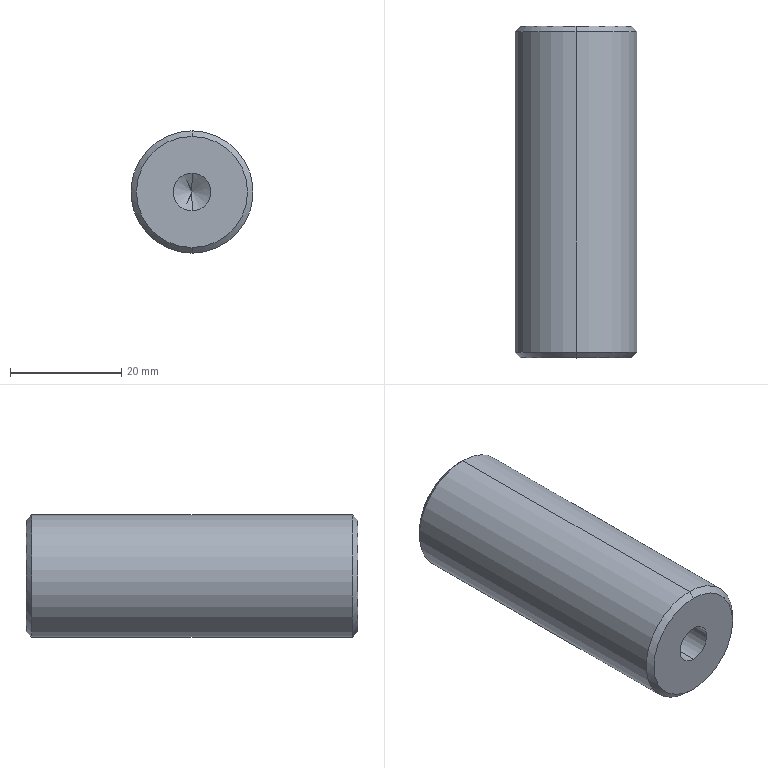Part | STEP file | circular post spca dia22-16-M8 | 1 solid | 16 faces | box 22 x 59.7 x 22 mm | volume 21361 mm3 | cone 8 | cylinder 6 | plane 2 | commonest cylinder face diameters 6.8 x4 22 x2
STEP:
#1=CARTESIAN_POINT('',(0.,0.,0.));
#2=DIRECTION('',(0.,0.,1.));
#3=DIRECTION('',(1.,0.,0.));
#4=AXIS2_PLACEMENT_3D('',#1,#2,#3);
#5=CARTESIAN_POINT('',(0.,0.,-10.));
#6=VERTEX_POINT('',#5);
#7=CARTESIAN_POINT('',(0.,0.,10.));
#8=VERTEX_POINT('',#7);
#9=CARTESIAN_POINT('',(0.,0.,0.));
#10=DIRECTION('',(0.,-1.,0.));
#11=DIRECTION('',(0.,0.,1.));
#12=AXIS2_PLACEMENT_3D('',#9,#10,#11);
#13=CIRCLE('',#12,10.);
#14=CARTESIAN_POINT('',(0.,1.,0.));
#15=DIRECTION('',(0.,1.,0.));
#16=DIRECTION('',(0.,0.,1.));
#17=AXIS2_PLACEMENT_3D('',#14,#15,#16);
#18=CONICAL_SURFACE('',#17,11.,0.7854);
#19=CARTESIAN_POINT('',(6.283,-1.));
#20=DIRECTION('',(-1.,0.));
#21=VECTOR('',#20,1.);
#22=LINE('',#19,#21);
#23=(GEOMETRIC_REPRESENTATION_CONTEXT(2)PARAMETRIC_REPRESENTATION_CONTEXT()REPRESENTATION_CONTEXT('',''));
#24=DEFINITIONAL_REPRESENTATION('',(#22),#23);
#25=PCURVE('',#18,#24);
#26=CARTESIAN_POINT('',(0.,0.,0.));
#27=DIRECTION('',(0.,1.,0.));
#28=DIRECTION('',(0.,0.,1.));
#29=AXIS2_PLACEMENT_3D('',#26,#27,#28);
#30=PLANE('',#29);
#31=CARTESIAN_POINT('',(10.,0.));
#32=CARTESIAN_POINT('',(10.,-17.321));
#33=CARTESIAN_POINT('',(-5.,-8.66));
#34=CARTESIAN_POINT('',(-20.,0.));
#35=CARTESIAN_POINT('',(-5.,8.66));
#36=CARTESIAN_POINT('',(10.,17.321));
#37=CARTESIAN_POINT('',(10.,0.));
#38=(BOUNDED_CURVE()B_SPLINE_CURVE(2,(#31,#32,#33,#34,#35,#36,#37),.UNSPECIFIED.,.T.,.F.)B_SPLINE_CURVE_WITH_KNOTS((1,2,2,2,2,1),(-2.094,0.,2.094,4.189,6.283,8.378),.UNSPECIFIED.)CURVE()GEOMETRIC_REPRESENTATION_ITEM()RATIONAL_B_SPLINE_CURVE((1.,0.5,1.,0.5,1.,0.5,1.))REPRESENTATION_ITEM(''));
#39=(GEOMETRIC_REPRESENTATION_CONTEXT(2)PARAMETRIC_REPRESENTATION_CONTEXT()REPRESENTATION_CONTEXT('',''));
#40=DEFINITIONAL_REPRESENTATION('',(#38),#39);
#41=PCURVE('',#30,#40);
#42=SURFACE_CURVE('',#13,(#25,#41),.PCURVE_S1.);
#43=EDGE_CURVE('',#6,#8,#42,.T.);
#44=ORIENTED_EDGE('',*,*,#43,.F.);
#45=CARTESIAN_POINT('',(0.,1.,-11.));
#46=VERTEX_POINT('',#45);
#47=CARTESIAN_POINT('',(0.,1.,-11.));
#48=DIRECTION('',(0.,0.7071,-0.7071));
#49=VECTOR('',#48,1.);
#50=LINE('',#47,#49);
#51=CARTESIAN_POINT('',(3.142,0.));
#52=DIRECTION('',(0.,1.));
#53=VECTOR('',#52,1.);
#54=LINE('',#51,#53);
#55=(GEOMETRIC_REPRESENTATION_CONTEXT(2)PARAMETRIC_REPRESENTATION_CONTEXT()REPRESENTATION_CONTEXT('',''));
#56=DEFINITIONAL_REPRESENTATION('',(#54),#55);
#57=PCURVE('',#18,#56);
#58=CARTESIAN_POINT('',(0.,1.,0.));
#59=DIRECTION('',(0.,1.,0.));
#60=DIRECTION('',(0.,0.,1.));
#61=AXIS2_PLACEMENT_3D('',#58,#59,#60);
#62=CONICAL_SURFACE('',#61,11.,0.7854);
#63=CARTESIAN_POINT('',(3.142,0.));
#64=DIRECTION('',(0.,1.));
#65=VECTOR('',#64,1.);
#66=LINE('',#63,#65);
#67=(GEOMETRIC_REPRESENTATION_CONTEXT(2)PARAMETRIC_REPRESENTATION_CONTEXT()REPRESENTATION_CONTEXT('',''));
#68=DEFINITIONAL_REPRESENTATION('',(#66),#67);
#69=PCURVE('',#62,#68);
#70=SURFACE_CURVE('',#50,(#57,#69),.PCURVE_S1.);
#71=EDGE_CURVE('',#6,#46,#70,.T.);
#72=ORIENTED_EDGE('',*,*,#71,.T.);
#73=CARTESIAN_POINT('',(0.,1.,11.));
#74=VERTEX_POINT('',#73);
#75=CARTESIAN_POINT('',(0.,1.,0.));
#76=DIRECTION('',(0.,1.,0.));
#77=DIRECTION('',(0.,0.,1.));
#78=AXIS2_PLACEMENT_3D('',#75,#76,#77);
#79=CIRCLE('',#78,11.);
#80=CARTESIAN_POINT('',(0.,0.));
#81=DIRECTION('',(1.,0.));
#82=VECTOR('',#81,1.);
#83=LINE('',#80,#82);
#84=(GEOMETRIC_REPRESENTATION_CONTEXT(2)PARAMETRIC_REPRESENTATION_CONTEXT()REPRESENTATION_CONTEXT('',''));
#85=DEFINITIONAL_REPRESENTATION('',(#83),#84);
#86=PCURVE('',#18,#85);
#87=CARTESIAN_POINT('',(0.,59.7,0.));
#88=DIRECTION('',(0.,-1.,0.));
#89=DIRECTION('',(0.,0.,-1.));
#90=AXIS2_PLACEMENT_3D('',#87,#88,#89);
#91=CYLINDRICAL_SURFACE('',#90,11.);
#92=CARTESIAN_POINT('',(3.142,58.7));
#93=DIRECTION('',(-1.,0.));
#94=VECTOR('',#93,1.);
#95=LINE('',#92,#94);
#96=(GEOMETRIC_REPRESENTATION_CONTEXT(2)PARAMETRIC_REPRESENTATION_CONTEXT()REPRESENTATION_CONTEXT('',''));
#97=DEFINITIONAL_REPRESENTATION('',(#95),#96);
#98=PCURVE('',#91,#97);
#99=SURFACE_CURVE('',#79,(#86,#98),.PCURVE_S1.);
#100=EDGE_CURVE('',#74,#46,#99,.T.);
#101=ORIENTED_EDGE('',*,*,#100,.F.);
#102=CARTESIAN_POINT('',(0.,1.,11.));
#103=DIRECTION('',(0.,0.7071,0.7071));
#104=VECTOR('',#103,1.);
#105=LINE('',#102,#104);
#106=CARTESIAN_POINT('',(0.,0.));
#107=DIRECTION('',(0.,1.));
#108=VECTOR('',#107,1.);
#109=LINE('',#106,#108);
#110=(GEOMETRIC_REPRESENTATION_CONTEXT(2)PARAMETRIC_REPRESENTATION_CONTEXT()REPRESENTATION_CONTEXT('',''));
#111=DEFINITIONAL_REPRESENTATION('',(#109),#110);
#112=PCURVE('',#18,#111);
#113=CARTESIAN_POINT('',(6.283,0.));
#114=DIRECTION('',(0.,1.));
#115=VECTOR('',#114,1.);
#116=LINE('',#113,#115);
#117=(GEOMETRIC_REPRESENTATION_CONTEXT(2)PARAMETRIC_REPRESENTATION_CONTEXT()REPRESENTATION_CONTEXT('',''));
#118=DEFINITIONAL_REPRESENTATION('',(#116),#117);
#119=PCURVE('',#62,#118);
#120=SURFACE_CURVE('',#105,(#112,#119),.PCURVE_S1.);
#121=EDGE_CURVE('',#8,#74,#120,.T.);
#122=ORIENTED_EDGE('',*,*,#121,.F.);
#123=EDGE_LOOP('',(#44,#72,#101,#122));
#124=FACE_BOUND('',#123,.T.);
#125=ADVANCED_FACE('',(#124),#18,.T.);
#126=CARTESIAN_POINT('',(0.,13.75,-3.4));
#127=VERTEX_POINT('',#126);
#128=CARTESIAN_POINT('',(0.,0.,-3.4));
#129=VERTEX_POINT('',#128);
#130=CARTESIAN_POINT('',(0.,-6.,-3.4));
#131=DIRECTION('',(0.,-1.,0.));
#132=VECTOR('',#131,1.);
#133=LINE('',#130,#132);
#134=CARTESIAN_POINT('',(0.,-6.,0.));
#135=DIRECTION('',(0.,-1.,0.));
#136=DIRECTION('',(0.,0.,-1.));
#137=AXIS2_PLACEMENT_3D('',#134,#135,#136);
#138=CYLINDRICAL_SURFACE('',#137,3.4);
#139=CARTESIAN_POINT('',(6.283,0.));
#140=DIRECTION('',(0.,1.));
#141=VECTOR('',#140,1.);
#142=LINE('',#139,#141);
#143=(GEOMETRIC_REPRESENTATION_CONTEXT(2)PARAMETRIC_REPRESENTATION_CONTEXT()REPRESENTATION_CONTEXT('',''));
#144=DEFINITIONAL_REPRESENTATION('',(#142),#143);
#145=PCURVE('',#138,#144);
#146=CARTESIAN_POINT('',(0.,-6.,0.));
#147=DIRECTION('',(0.,-1.,0.));
#148=DIRECTION('',(0.,0.,-1.));
#149=AXIS2_PLACEMENT_3D('',#146,#147,#148);
#150=CYLINDRICAL_SURFACE('',#149,3.4);
#151=CARTESIAN_POINT('',(0.,0.));
#152=DIRECTION('',(0.,1.));
#153=VECTOR('',#152,1.);
#154=LINE('',#151,#153);
#155=(GEOMETRIC_REPRESENTATION_CONTEXT(2)PARAMETRIC_REPRESENTATION_CONTEXT()REPRESENTATION_CONTEXT('',''));
#156=DEFINITIONAL_REPRESENTATION('',(#154),#155);
#157=PCURVE('',#150,#156);
#158=SURFACE_CURVE('',#133,(#145,#157),.PCURVE_S1.);
#159=EDGE_CURVE('',#127,#129,#158,.T.);
#160=ORIENTED_EDGE('',*,*,#159,.T.);
#161=CARTESIAN_POINT('',(0.,0.,3.4));
#162=VERTEX_POINT('',#161);
#163=CARTESIAN_POINT('',(0.,0.,0.));
#164=DIRECTION('',(0.,1.,0.));
#165=DIRECTION('',(0.,0.,-1.));
#166=AXIS2_PLACEMENT_3D('',#163,#164,#165);
#167=CIRCLE('',#166,3.4);
#168=CARTESIAN_POINT('',(6.283,-6.));
#169=DIRECTION('',(-1.,0.));
#170=VECTOR('',#169,1.);
#171=LINE('',#168,#170);
#172=(GEOMETRIC_REPRESENTATION_CONTEXT(2)PARAMETRIC_REPRESENTATION_CONTEXT()REPRESENTATION_CONTEXT('',''));
#173=DEFINITIONAL_REPRESENTATION('',(#171),#172);
#174=PCURVE('',#138,#173);
#175=CARTESIAN_POINT('',(0.,0.));
#176=DIRECTION('',(-1.,0.));
#177=AXIS2_PLACEMENT_2D('',#175,#176);
#178=CIRCLE('',#177,3.4);
#179=(GEOMETRIC_REPRESENTATION_CONTEXT(2)PARAMETRIC_REPRESENTATION_CONTEXT()REPRESENTATION_CONTEXT('',''));
#180=DEFINITIONAL_REPRESENTATION('',(#178),#179);
#181=PCURVE('',#30,#180);
#182=SURFACE_CURVE('',#167,(#174,#181),.PCURVE_S1.);
#183=EDGE_CURVE('',#129,#162,#182,.T.);
#184=ORIENTED_EDGE('',*,*,#183,.T.);
#185=CARTESIAN_POINT('',(0.,13.75,3.4));
#186=VERTEX_POINT('',#185);
#187=CARTESIAN_POINT('',(0.,-6.,3.4));
#188=DIRECTION('',(0.,-1.,0.));
#189=VECTOR('',#188,1.);
#190=LINE('',#187,#189);
#191=CARTESIAN_POINT('',(3.142,0.));
#192=DIRECTION('',(0.,1.));
#193=VECTOR('',#192,1.);
#194=LINE('',#191,#193);
#195=(GEOMETRIC_REPRESENTATION_CONTEXT(2)PARAMETRIC_REPRESENTATION_CONTEXT()REPRESENTATION_CONTEXT('',''));
#196=DEFINITIONAL_REPRESENTATION('',(#194),#195);
#197=PCURVE('',#138,#196);
#198=CARTESIAN_POINT('',(3.142,0.));
#199=DIRECTION('',(0.,1.));
#200=VECTOR('',#199,1.);
#201=LINE('',#198,#200);
#202=(GEOMETRIC_REPRESENTATION_CONTEXT(2)PARAMETRIC_REPRESENTATION_CONTEXT()REPRESENTATION_CONTEXT('',''));
#203=DEFINITIONAL_REPRESENTATION('',(#201),#202);
#204=PCURVE('',#150,#203);
#205=SURFACE_CURVE('',#190,(#197,#204),.PCURVE_S1.);
#206=EDGE_CURVE('',#186,#162,#205,.T.);
#207=ORIENTED_EDGE('',*,*,#206,.F.);
#208=CARTESIAN_POINT('',(0.,13.75,0.));
#209=DIRECTION('',(0.,-1.,0.));
#210=DIRECTION('',(0.,0.,-1.));
#211=AXIS2_PLACEMENT_3D('',#208,#209,#210);
#212=CIRCLE('',#211,3.4);
#213=CARTESIAN_POINT('',(0.,-19.75));
#214=DIRECTION('',(1.,0.));
#215=VECTOR('',#214,1.);
#216=LINE('',#213,#215);
#217=(GEOMETRIC_REPRESENTATION_CONTEXT(2)PARAMETRIC_REPRESENTATION_CONTEXT()REPRESENTATION_CONTEXT('',''));
#218=DEFINITIONAL_REPRESENTATION('',(#216),#217);
#219=PCURVE('',#138,#218);
#220=CARTESIAN_POINT('',(0.,13.75,0.));
#221=DIRECTION('',(0.,-1.,0.));
#222=DIRECTION('',(0.,0.,-1.));
#223=AXIS2_PLACEMENT_3D('',#220,#221,#222);
#224=CONICAL_SURFACE('',#223,3.4,1.03);
#225=CARTESIAN_POINT('',(0.,0.));
#226=DIRECTION('',(1.,0.));
#227=VECTOR('',#226,1.);
#228=LINE('',#225,#227);
#229=(GEOMETRIC_REPRESENTATION_CONTEXT(2)PARAMETRIC_REPRESENTATION_CONTEXT()REPRESENTATION_CONTEXT('',''));
#230=DEFINITIONAL_REPRESENTATION('',(#228),#229);
#231=PCURVE('',#224,#230);
#232=SURFACE_CURVE('',#212,(#219,#231),.PCURVE_S1.);
#233=EDGE_CURVE('',#186,#127,#232,.T.);
#234=ORIENTED_EDGE('',*,*,#233,.T.);
#235=EDGE_LOOP('',(#160,#184,#207,#234));
#236=FACE_BOUND('',#235,.F.);
#237=ADVANCED_FACE('',(#236),#138,.F.);
#238=ORIENTED_EDGE('',*,*,#233,.F.);
#239=CARTESIAN_POINT('',(0.,15.793,0.));
#240=VERTEX_POINT('',#239);
#241=CARTESIAN_POINT('',(0.,13.75,3.4));
#242=DIRECTION('',(0.,-0.515,0.8572));
#243=VECTOR('',#242,1.);
#244=LINE('',#241,#243);
#245=CARTESIAN_POINT('',(3.142,0.));
#246=DIRECTION('',(0.,1.));
#247=VECTOR('',#246,1.);
#248=LINE('',#245,#247);
#249=(GEOMETRIC_REPRESENTATION_CONTEXT(2)PARAMETRIC_REPRESENTATION_CONTEXT()REPRESENTATION_CONTEXT('',''));
#250=DEFINITIONAL_REPRESENTATION('',(#248),#249);
#251=PCURVE('',#224,#250);
#252=CARTESIAN_POINT('',(0.,13.75,0.));
#253=DIRECTION('',(0.,-1.,0.));
#254=DIRECTION('',(0.,0.,-1.));
#255=AXIS2_PLACEMENT_3D('',#252,#253,#254);
#256=CONICAL_SURFACE('',#255,3.4,1.03);
#257=CARTESIAN_POINT('',(3.142,0.));
#258=DIRECTION('',(0.,1.));
#259=VECTOR('',#258,1.);
#260=LINE('',#257,#259);
#261=(GEOMETRIC_REPRESENTATION_CONTEXT(2)PARAMETRIC_REPRESENTATION_CONTEXT()REPRESENTATION_CONTEXT('',''));
#262=DEFINITIONAL_REPRESENTATION('',(#260),#261);
#263=PCURVE('',#256,#262);
#264=SURFACE_CURVE('',#244,(#251,#263),.PCURVE_S1.);
#265=EDGE_CURVE('',#240,#186,#264,.T.);
#266=ORIENTED_EDGE('',*,*,#265,.F.);
#267=CARTESIAN_POINT('',(0.,13.75,-3.4));
#268=DIRECTION('',(0.,-0.515,-0.8572));
#269=VECTOR('',#268,1.);
#270=LINE('',#267,#269);
#271=CARTESIAN_POINT('',(6.283,0.));
#272=DIRECTION('',(0.,1.));
#273=VECTOR('',#272,1.);
#274=LINE('',#271,#273);
#275=(GEOMETRIC_REPRESENTATION_CONTEXT(2)PARAMETRIC_REPRESENTATION_CONTEXT()REPRESENTATION_CONTEXT('',''));
#276=DEFINITIONAL_REPRESENTATION('',(#274),#275);
#277=PCURVE('',#224,#276);
#278=CARTESIAN_POINT('',(0.,0.));
#279=DIRECTION('',(0.,1.));
#280=VECTOR('',#279,1.);
#281=LINE('',#278,#280);
#282=(GEOMETRIC_REPRESENTATION_CONTEXT(2)PARAMETRIC_REPRESENTATION_CONTEXT()REPRESENTATION_CONTEXT('',''));
#283=DEFINITIONAL_REPRESENTATION('',(#281),#282);
#284=PCURVE('',#256,#283);
#285=SURFACE_CURVE('',#270,(#277,#284),.PCURVE_S1.);
#286=EDGE_CURVE('',#240,#127,#285,.T.);
#287=ORIENTED_EDGE('',*,*,#286,.T.);
#288=EDGE_LOOP('',(#238,#266,#287));
#289=FACE_BOUND('',#288,.F.);
#290=ADVANCED_FACE('',(#289),#224,.F.);
#291=CARTESIAN_POINT('',(0.,39.95,3.4));
#292=VERTEX_POINT('',#291);
#293=CARTESIAN_POINT('',(0.,59.7,3.4));
#294=VERTEX_POINT('',#293);
#295=CARTESIAN_POINT('',(0.,59.7,3.4));
#296=DIRECTION('',(0.,1.,0.));
#297=VECTOR('',#296,1.);
#298=LINE('',#295,#297);
#299=CARTESIAN_POINT('',(0.,59.7,0.));
#300=DIRECTION('',(0.,1.,0.));
#301=DIRECTION('',(0.,0.,1.));
#302=AXIS2_PLACEMENT_3D('',#299,#300,#301);
#303=CYLINDRICAL_SURFACE('',#302,3.4);
#304=CARTESIAN_POINT('',(6.283,0.));
#305=DIRECTION('',(0.,1.));
#306=VECTOR('',#305,1.);
#307=LINE('',#304,#306);
#308=(GEOMETRIC_REPRESENTATION_CONTEXT(2)PARAMETRIC_REPRESENTATION_CONTEXT()REPRESENTATION_CONTEXT('',''));
#309=DEFINITIONAL_REPRESENTATION('',(#307),#308);
#310=PCURVE('',#303,#309);
#311=CARTESIAN_POINT('',(0.,59.7,0.));
#312=DIRECTION('',(0.,1.,0.));
#313=DIRECTION('',(0.,0.,1.));
#314=AXIS2_PLACEMENT_3D('',#311,#312,#313);
#315=CYLINDRICAL_SURFACE('',#314,3.4);
#316=CARTESIAN_POINT('',(0.,0.));
#317=DIRECTION('',(0.,1.));
#318=VECTOR('',#317,1.);
#319=LINE('',#316,#318);
#320=(GEOMETRIC_REPRESENTATION_CONTEXT(2)PARAMETRIC_REPRESENTATION_CONTEXT()REPRESENTATION_CONTEXT('',''));
#321=DEFINITIONAL_REPRESENTATION('',(#319),#320);
#322=PCURVE('',#315,#321);
#323=SURFACE_CURVE('',#298,(#310,#322),.PCURVE_S1.);
#324=EDGE_CURVE('',#292,#294,#323,.T.);
#325=ORIENTED_EDGE('',*,*,#324,.T.);
#326=CARTESIAN_POINT('',(0.,59.7,-3.4));
#327=VERTEX_POINT('',#326);
#328=CARTESIAN_POINT('',(0.,59.7,0.));
#329=DIRECTION('',(0.,1.,0.));
#330=DIRECTION('',(0.,0.,1.));
#331=AXIS2_PLACEMENT_3D('',#328,#329,#330);
#332=CIRCLE('',#331,3.4);
#333=CARTESIAN_POINT('',(0.,0.));
#334=DIRECTION('',(1.,0.));
#335=VECTOR('',#334,1.);
#336=LINE('',#333,#335);
#337=(GEOMETRIC_REPRESENTATION_CONTEXT(2)PARAMETRIC_REPRESENTATION_CONTEXT()REPRESENTATION_CONTEXT('',''));
#338=DEFINITIONAL_REPRESENTATION('',(#336),#337);
#339=PCURVE('',#303,#338);
#340=CARTESIAN_POINT('',(0.,59.7,0.));
#341=DIRECTION('',(0.,1.,0.));
#342=DIRECTION('',(0.,0.,1.));
#343=AXIS2_PLACEMENT_3D('',#340,#341,#342);
#344=PLANE('',#343);
#345=CARTESIAN_POINT('',(0.,0.));
#346=DIRECTION('',(1.,0.));
#347=AXIS2_PLACEMENT_2D('',#345,#346);
#348=CIRCLE('',#347,3.4);
#349=(GEOMETRIC_REPRESENTATION_CONTEXT(2)PARAMETRIC_REPRESENTATION_CONTEXT()REPRESENTATION_CONTEXT('',''));
#350=DEFINITIONAL_REPRESENTATION('',(#348),#349);
#351=PCURVE('',#344,#350);
#352=SURFACE_CURVE('',#332,(#339,#351),.PCURVE_S1.);
#353=EDGE_CURVE('',#327,#294,#352,.T.);
#354=ORIENTED_EDGE('',*,*,#353,.F.);
#355=CARTESIAN_POINT('',(0.,39.95,-3.4));
#356=VERTEX_POINT('',#355);
#357=CARTESIAN_POINT('',(0.,59.7,-3.4));
#358=DIRECTION('',(0.,1.,0.));
#359=VECTOR('',#358,1.);
#360=LINE('',#357,#359);
#361=CARTESIAN_POINT('',(3.142,0.));
#362=DIRECTION('',(0.,1.));
#363=VECTOR('',#362,1.);
#364=LINE('',#361,#363);
#365=(GEOMETRIC_REPRESENTATION_CONTEXT(2)PARAMETRIC_REPRESENTATION_CONTEXT()REPRESENTATION_CONTEXT('',''));
#366=DEFINITIONAL_REPRESENTATION('',(#364),#365);
#367=PCURVE('',#303,#366);
#368=CARTESIAN_POINT('',(3.142,0.));
#369=DIRECTION('',(0.,1.));
#370=VECTOR('',#369,1.);
#371=LINE('',#368,#370);
#372=(GEOMETRIC_REPRESENTATION_CONTEXT(2)PARAMETRIC_REPRESENTATION_CONTEXT()REPRESENTATION_CONTEXT('',''));
#373=DEFINITIONAL_REPRESENTATION('',(#371),#372);
#374=PCURVE('',#315,#373);
#375=SURFACE_CURVE('',#360,(#367,#374),.PCURVE_S1.);
#376=EDGE_CURVE('',#356,#327,#375,.T.);
#377=ORIENTED_EDGE('',*,*,#376,.F.);
#378=CARTESIAN_POINT('',(0.,39.95,0.));
#379=DIRECTION('',(0.,1.,0.));
#380=DIRECTION('',(0.,0.,1.));
#381=AXIS2_PLACEMENT_3D('',#378,#379,#380);
#382=CIRCLE('',#381,3.4);
#383=CARTESIAN_POINT('',(0.,-19.75));
#384=DIRECTION('',(1.,0.));
#385=VECTOR('',#384,1.);
#386=LINE('',#383,#385);
#387=(GEOMETRIC_REPRESENTATION_CONTEXT(2)PARAMETRIC_REPRESENTATION_CONTEXT()REPRESENTATION_CONTEXT('',''));
#388=DEFINITIONAL_REPRESENTATION('',(#386),#387);
#389=PCURVE('',#303,#388);
#390=CARTESIAN_POINT('',(0.,39.95,0.));
#391=DIRECTION('',(0.,1.,0.));
#392=DIRECTION('',(0.,0.,1.));
#393=AXIS2_PLACEMENT_3D('',#390,#391,#392);
#394=CONICAL_SURFACE('',#393,3.4,1.03);
#395=CARTESIAN_POINT('',(0.,0.));
#396=DIRECTION('',(1.,0.));
#397=VECTOR('',#396,1.);
#398=LINE('',#395,#397);
#399=(GEOMETRIC_REPRESENTATION_CONTEXT(2)PARAMETRIC_REPRESENTATION_CONTEXT()REPRESENTATION_CONTEXT('',''));
#400=DEFINITIONAL_REPRESENTATION('',(#398),#399);
#401=PCURVE('',#394,#400);
#402=SURFACE_CURVE('',#382,(#389,#401),.PCURVE_S1.);
#403=EDGE_CURVE('',#356,#292,#402,.T.);
#404=ORIENTED_EDGE('',*,*,#403,.T.);
#405=EDGE_LOOP('',(#325,#354,#377,#404));
#406=FACE_BOUND('',#405,.F.);
#407=ADVANCED_FACE('',(#406),#303,.F.);
#408=ORIENTED_EDGE('',*,*,#403,.F.);
#409=CARTESIAN_POINT('',(0.,37.907,0.));
#410=VERTEX_POINT('',#409);
#411=CARTESIAN_POINT('',(0.,39.95,-3.4));
#412=DIRECTION('',(0.,0.515,-0.8572));
#413=VECTOR('',#412,1.);
#414=LINE('',#411,#413);
#415=CARTESIAN_POINT('',(3.142,0.));
#416=DIRECTION('',(0.,1.));
#417=VECTOR('',#416,1.);
#418=LINE('',#415,#417);
#419=(GEOMETRIC_REPRESENTATION_CONTEXT(2)PARAMETRIC_REPRESENTATION_CONTEXT()REPRESENTATION_CONTEXT('',''));
#420=DEFINITIONAL_REPRESENTATION('',(#418),#419);
#421=PCURVE('',#394,#420);
#422=CARTESIAN_POINT('',(0.,39.95,0.));
#423=DIRECTION('',(0.,1.,0.));
#424=DIRECTION('',(0.,0.,1.));
#425=AXIS2_PLACEMENT_3D('',#422,#423,#424);
#426=CONICAL_SURFACE('',#425,3.4,1.03);
#427=CARTESIAN_POINT('',(3.142,0.));
#428=DIRECTION('',(0.,1.));
#429=VECTOR('',#428,1.);
#430=LINE('',#427,#429);
#431=(GEOMETRIC_REPRESENTATION_CONTEXT(2)PARAMETRIC_REPRESENTATION_CONTEXT()REPRESENTATION_CONTEXT('',''));
#432=DEFINITIONAL_REPRESENTATION('',(#430),#431);
#433=PCURVE('',#426,#432);
#434=SURFACE_CURVE('',#414,(#421,#433),.PCURVE_S1.);
#435=EDGE_CURVE('',#410,#356,#434,.T.);
#436=ORIENTED_EDGE('',*,*,#435,.F.);
#437=CARTESIAN_POINT('',(0.,39.95,3.4));
#438=DIRECTION('',(0.,0.515,0.8572));
#439=VECTOR('',#438,1.);
#440=LINE('',#437,#439);
#441=CARTESIAN_POINT('',(6.283,0.));
#442=DIRECTION('',(0.,1.));
#443=VECTOR('',#442,1.);
#444=LINE('',#441,#443);
#445=(GEOMETRIC_REPRESENTATION_CONTEXT(2)PARAMETRIC_REPRESENTATION_CONTEXT()REPRESENTATION_CONTEXT('',''));
#446=DEFINITIONAL_REPRESENTATION('',(#444),#445);
#447=PCURVE('',#394,#446);
#448=CARTESIAN_POINT('',(0.,0.));
#449=DIRECTION('',(0.,1.));
#450=VECTOR('',#449,1.);
#451=LINE('',#448,#450);
#452=(GEOMETRIC_REPRESENTATION_CONTEXT(2)PARAMETRIC_REPRESENTATION_CONTEXT()REPRESENTATION_CONTEXT('',''));
#453=DEFINITIONAL_REPRESENTATION('',(#451),#452);
#454=PCURVE('',#426,#453);
#455=SURFACE_CURVE('',#440,(#447,#454),.PCURVE_S1.);
#456=EDGE_CURVE('',#410,#292,#455,.T.);
#457=ORIENTED_EDGE('',*,*,#456,.T.);
#458=EDGE_LOOP('',(#408,#436,#457));
#459=FACE_BOUND('',#458,.F.);
#460=ADVANCED_FACE('',(#459),#394,.F.);
#461=CARTESIAN_POINT('',(0.,59.7,10.));
#462=VERTEX_POINT('',#461);
#463=CARTESIAN_POINT('',(0.,59.7,-10.));
#464=VERTEX_POINT('',#463);
#465=CARTESIAN_POINT('',(0.,59.7,0.));
#466=DIRECTION('',(0.,1.,0.));
#467=DIRECTION('',(0.,0.,1.));
#468=AXIS2_PLACEMENT_3D('',#465,#466,#467);
#469=CIRCLE('',#468,10.);
#470=CARTESIAN_POINT('',(0.,59.7,0.));
#471=DIRECTION('',(0.,-1.,0.));
#472=DIRECTION('',(0.,0.,-1.));
#473=AXIS2_PLACEMENT_3D('',#470,#471,#472);
#474=CONICAL_SURFACE('',#473,10.,0.7854);
#475=CARTESIAN_POINT('',(3.142,0.));
#476=DIRECTION('',(-1.,0.));
#477=VECTOR('',#476,1.);
#478=LINE('',#475,#477);
#479=(GEOMETRIC_REPRESENTATION_CONTEXT(2)PARAMETRIC_REPRESENTATION_CONTEXT()REPRESENTATION_CONTEXT('',''));
#480=DEFINITIONAL_REPRESENTATION('',(#478),#479);
#481=PCURVE('',#474,#480);
#482=CARTESIAN_POINT('',(0.,0.));
#483=DIRECTION('',(1.,0.));
#484=AXIS2_PLACEMENT_2D('',#482,#483);
#485=CIRCLE('',#484,10.);
#486=(GEOMETRIC_REPRESENTATION_CONTEXT(2)PARAMETRIC_REPRESENTATION_CONTEXT()REPRESENTATION_CONTEXT('',''));
#487=DEFINITIONAL_REPRESENTATION('',(#485),#486);
#488=PCURVE('',#344,#487);
#489=SURFACE_CURVE('',#469,(#481,#488),.PCURVE_S1.);
#490=EDGE_CURVE('',#462,#464,#489,.T.);
#491=ORIENTED_EDGE('',*,*,#490,.F.);
#492=CARTESIAN_POINT('',(0.,58.7,11.));
#493=VERTEX_POINT('',#492);
#494=CARTESIAN_POINT('',(0.,59.7,10.));
#495=DIRECTION('',(0.,-0.7071,0.7071));
#496=VECTOR('',#495,1.);
#497=LINE('',#494,#496);
#498=CARTESIAN_POINT('',(3.142,0.));
#499=DIRECTION('',(0.,1.));
#500=VECTOR('',#499,1.);
#501=LINE('',#498,#500);
#502=(GEOMETRIC_REPRESENTATION_CONTEXT(2)PARAMETRIC_REPRESENTATION_CONTEXT()REPRESENTATION_CONTEXT('',''));
#503=DEFINITIONAL_REPRESENTATION('',(#501),#502);
#504=PCURVE('',#474,#503);
#505=CARTESIAN_POINT('',(0.,59.7,0.));
#506=DIRECTION('',(0.,-1.,0.));
#507=DIRECTION('',(0.,0.,-1.));
#508=AXIS2_PLACEMENT_3D('',#505,#506,#507);
#509=CONICAL_SURFACE('',#508,10.,0.7854);
#510=CARTESIAN_POINT('',(3.142,0.));
#511=DIRECTION('',(0.,1.));
#512=VECTOR('',#511,1.);
#513=LINE('',#510,#512);
#514=(GEOMETRIC_REPRESENTATION_CONTEXT(2)PARAMETRIC_REPRESENTATION_CONTEXT()REPRESENTATION_CONTEXT('',''));
#515=DEFINITIONAL_REPRESENTATION('',(#513),#514);
#516=PCURVE('',#509,#515);
#517=SURFACE_CURVE('',#497,(#504,#516),.PCURVE_S1.);
#518=EDGE_CURVE('',#462,#493,#517,.T.);
#519=ORIENTED_EDGE('',*,*,#518,.T.);
#520=CARTESIAN_POINT('',(0.,58.7,-11.));
#521=VERTEX_POINT('',#520);
#522=CARTESIAN_POINT('',(0.,58.7,0.));
#523=DIRECTION('',(0.,-1.,0.));
#524=DIRECTION('',(0.,0.,1.));
#525=AXIS2_PLACEMENT_3D('',#522,#523,#524);
#526=CIRCLE('',#525,11.);
#527=CARTESIAN_POINT('',(-3.142,1.));
#528=DIRECTION('',(1.,0.));
#529=VECTOR('',#528,1.);
#530=LINE('',#527,#529);
#531=(GEOMETRIC_REPRESENTATION_CONTEXT(2)PARAMETRIC_REPRESENTATION_CONTEXT()REPRESENTATION_CONTEXT('',''));
#532=DEFINITIONAL_REPRESENTATION('',(#530),#531);
#533=PCURVE('',#474,#532);
#534=CARTESIAN_POINT('',(-3.142,1.));
#535=DIRECTION('',(1.,0.));
#536=VECTOR('',#535,1.);
#537=LINE('',#534,#536);
#538=(GEOMETRIC_REPRESENTATION_CONTEXT(2)PARAMETRIC_REPRESENTATION_CONTEXT()REPRESENTATION_CONTEXT('',''));
#539=DEFINITIONAL_REPRESENTATION('',(#537),#538);
#540=PCURVE('',#91,#539);
#541=SURFACE_CURVE('',#526,(#533,#540),.PCURVE_S1.);
#542=EDGE_CURVE('',#521,#493,#541,.T.);
#543=ORIENTED_EDGE('',*,*,#542,.F.);
#544=CARTESIAN_POINT('',(0.,59.7,-10.));
#545=DIRECTION('',(0.,-0.7071,-0.7071));
#546=VECTOR('',#545,1.);
#547=LINE('',#544,#546);
#548=CARTESIAN_POINT('',(0.,0.));
#549=DIRECTION('',(0.,1.));
#550=VECTOR('',#549,1.);
#551=LINE('',#548,#550);
#552=(GEOMETRIC_REPRESENTATION_CONTEXT(2)PARAMETRIC_REPRESENTATION_CONTEXT()REPRESENTATION_CONTEXT('',''));
#553=DEFINITIONAL_REPRESENTATION('',(#551),#552);
#554=PCURVE('',#474,#553);
#555=CARTESIAN_POINT('',(6.283,0.));
#556=DIRECTION('',(0.,1.));
#557=VECTOR('',#556,1.);
#558=LINE('',#555,#557);
#559=(GEOMETRIC_REPRESENTATION_CONTEXT(2)PARAMETRIC_REPRESENTATION_CONTEXT()REPRESENTATION_CONTEXT('',''));
#560=DEFINITIONAL_REPRESENTATION('',(#558),#559);
#561=PCURVE('',#509,#560);
#562=SURFACE_CURVE('',#547,(#554,#561),.PCURVE_S1.);
#563=EDGE_CURVE('',#464,#521,#562,.T.);
#564=ORIENTED_EDGE('',*,*,#563,.F.);
#565=EDGE_LOOP('',(#491,#519,#543,#564));
#566=FACE_BOUND('',#565,.T.);
#567=ADVANCED_FACE('',(#566),#474,.T.);
#568=ORIENTED_EDGE('',*,*,#542,.T.);
#569=CARTESIAN_POINT('',(0.,59.7,11.));
#570=DIRECTION('',(0.,-1.,0.));
#571=VECTOR('',#570,1.);
#572=LINE('',#569,#571);
#573=CARTESIAN_POINT('',(3.142,0.));
#574=DIRECTION('',(0.,1.));
#575=VECTOR('',#574,1.);
#576=LINE('',#573,#575);
#577=(GEOMETRIC_REPRESENTATION_CONTEXT(2)PARAMETRIC_REPRESENTATION_CONTEXT()REPRESENTATION_CONTEXT('',''));
#578=DEFINITIONAL_REPRESENTATION('',(#576),#577);
#579=PCURVE('',#91,#578);
#580=CARTESIAN_POINT('',(0.,59.7,0.));
#581=DIRECTION('',(0.,-1.,0.));
#582=DIRECTION('',(0.,0.,-1.));
#583=AXIS2_PLACEMENT_3D('',#580,#581,#582);
#584=CYLINDRICAL_SURFACE('',#583,11.);
#585=CARTESIAN_POINT('',(3.142,0.));
#586=DIRECTION('',(0.,1.));
#587=VECTOR('',#586,1.);
#588=LINE('',#585,#587);
#589=(GEOMETRIC_REPRESENTATION_CONTEXT(2)PARAMETRIC_REPRESENTATION_CONTEXT()REPRESENTATION_CONTEXT('',''));
#590=DEFINITIONAL_REPRESENTATION('',(#588),#589);
#591=PCURVE('',#584,#590);
#592=SURFACE_CURVE('',#572,(#579,#591),.PCURVE_S1.);
#593=EDGE_CURVE('',#493,#74,#592,.T.);
#594=ORIENTED_EDGE('',*,*,#593,.T.);
#595=ORIENTED_EDGE('',*,*,#100,.T.);
#596=CARTESIAN_POINT('',(0.,59.7,-11.));
#597=DIRECTION('',(0.,-1.,0.));
#598=VECTOR('',#597,1.);
#599=LINE('',#596,#598);
#600=CARTESIAN_POINT('',(0.,0.));
#601=DIRECTION('',(0.,1.));
#602=VECTOR('',#601,1.);
#603=LINE('',#600,#602);
#604=(GEOMETRIC_REPRESENTATION_CONTEXT(2)PARAMETRIC_REPRESENTATION_CONTEXT()REPRESENTATION_CONTEXT('',''));
#605=DEFINITIONAL_REPRESENTATION('',(#603),#604);
#606=PCURVE('',#91,#605);
#607=CARTESIAN_POINT('',(6.283,0.));
#608=DIRECTION('',(0.,1.));
#609=VECTOR('',#608,1.);
#610=LINE('',#607,#609);
#611=(GEOMETRIC_REPRESENTATION_CONTEXT(2)PARAMETRIC_REPRESENTATION_CONTEXT()REPRESENTATION_CONTEXT('',''));
#612=DEFINITIONAL_REPRESENTATION('',(#610),#611);
#613=PCURVE('',#584,#612);
#614=SURFACE_CURVE('',#599,(#606,#613),.PCURVE_S1.);
#615=EDGE_CURVE('',#521,#46,#614,.T.);
#616=ORIENTED_EDGE('',*,*,#615,.F.);
#617=EDGE_LOOP('',(#568,#594,#595,#616));
#618=FACE_BOUND('',#617,.T.);
#619=ADVANCED_FACE('',(#618),#91,.T.);
#620=CARTESIAN_POINT('',(0.,0.,0.));
#621=DIRECTION('',(0.,-1.,0.));
#622=DIRECTION('',(0.,0.,1.));
#623=AXIS2_PLACEMENT_3D('',#620,#621,#622);
#624=CIRCLE('',#623,10.);
#625=CARTESIAN_POINT('',(10.,0.));
#626=CARTESIAN_POINT('',(10.,-17.321));
#627=CARTESIAN_POINT('',(-5.,-8.66));
#628=CARTESIAN_POINT('',(-20.,0.));
#629=CARTESIAN_POINT('',(-5.,8.66));
#630=CARTESIAN_POINT('',(10.,17.321));
#631=CARTESIAN_POINT('',(10.,0.));
#632=(BOUNDED_CURVE()B_SPLINE_CURVE(2,(#625,#626,#627,#628,#629,#630,#631),.UNSPECIFIED.,.T.,.F.)B_SPLINE_CURVE_WITH_KNOTS((1,2,2,2,2,1),(-2.094,0.,2.094,4.189,6.283,8.378),.UNSPECIFIED.)CURVE()GEOMETRIC_REPRESENTATION_ITEM()RATIONAL_B_SPLINE_CURVE((1.,0.5,1.,0.5,1.,0.5,1.))REPRESENTATION_ITEM(''));
#633=(GEOMETRIC_REPRESENTATION_CONTEXT(2)PARAMETRIC_REPRESENTATION_CONTEXT()REPRESENTATION_CONTEXT('',''));
#634=DEFINITIONAL_REPRESENTATION('',(#632),#633);
#635=PCURVE('',#30,#634);
#636=CARTESIAN_POINT('',(6.283,-1.));
#637=DIRECTION('',(-1.,0.));
#638=VECTOR('',#637,1.);
#639=LINE('',#636,#638);
#640=(GEOMETRIC_REPRESENTATION_CONTEXT(2)PARAMETRIC_REPRESENTATION_CONTEXT()REPRESENTATION_CONTEXT('',''));
#641=DEFINITIONAL_REPRESENTATION('',(#639),#640);
#642=PCURVE('',#62,#641);
#643=SURFACE_CURVE('',#624,(#635,#642),.PCURVE_S1.);
#644=EDGE_CURVE('',#8,#6,#643,.T.);
#645=ORIENTED_EDGE('',*,*,#644,.T.);
#646=ORIENTED_EDGE('',*,*,#43,.T.);
#647=EDGE_LOOP('',(#645,#646));
#648=FACE_BOUND('',#647,.T.);
#649=ORIENTED_EDGE('',*,*,#183,.T.);
#650=CARTESIAN_POINT('',(0.,0.,0.));
#651=DIRECTION('',(0.,1.,0.));
#652=DIRECTION('',(0.,0.,-1.));
#653=AXIS2_PLACEMENT_3D('',#650,#651,#652);
#654=CIRCLE('',#653,3.4);
#655=CARTESIAN_POINT('',(0.,0.));
#656=DIRECTION('',(-1.,0.));
#657=AXIS2_PLACEMENT_2D('',#655,#656);
#658=CIRCLE('',#657,3.4);
#659=(GEOMETRIC_REPRESENTATION_CONTEXT(2)PARAMETRIC_REPRESENTATION_CONTEXT()REPRESENTATION_CONTEXT('',''));
#660=DEFINITIONAL_REPRESENTATION('',(#658),#659);
#661=PCURVE('',#30,#660);
#662=CARTESIAN_POINT('',(6.283,-6.));
#663=DIRECTION('',(-1.,0.));
#664=VECTOR('',#663,1.);
#665=LINE('',#662,#664);
#666=(GEOMETRIC_REPRESENTATION_CONTEXT(2)PARAMETRIC_REPRESENTATION_CONTEXT()REPRESENTATION_CONTEXT('',''));
#667=DEFINITIONAL_REPRESENTATION('',(#665),#666);
#668=PCURVE('',#150,#667);
#669=SURFACE_CURVE('',#654,(#661,#668),.PCURVE_S1.);
#670=EDGE_CURVE('',#162,#129,#669,.T.);
#671=ORIENTED_EDGE('',*,*,#670,.T.);
#672=EDGE_LOOP('',(#649,#671));
#673=FACE_BOUND('',#672,.T.);
#674=ADVANCED_FACE('',(#648,#673),#30,.F.);
#675=ORIENTED_EDGE('',*,*,#593,.F.);
#676=CARTESIAN_POINT('',(0.,58.7,0.));
#677=DIRECTION('',(0.,-1.,0.));
#678=DIRECTION('',(0.,0.,1.));
#679=AXIS2_PLACEMENT_3D('',#676,#677,#678);
#680=CIRCLE('',#679,11.);
#681=CARTESIAN_POINT('',(3.142,1.));
#682=DIRECTION('',(1.,0.));
#683=VECTOR('',#682,1.);
#684=LINE('',#681,#683);
#685=(GEOMETRIC_REPRESENTATION_CONTEXT(2)PARAMETRIC_REPRESENTATION_CONTEXT()REPRESENTATION_CONTEXT('',''));
#686=DEFINITIONAL_REPRESENTATION('',(#684),#685);
#687=PCURVE('',#584,#686);
#688=CARTESIAN_POINT('',(3.142,1.));
#689=DIRECTION('',(1.,0.));
#690=VECTOR('',#689,1.);
#691=LINE('',#688,#690);
#692=(GEOMETRIC_REPRESENTATION_CONTEXT(2)PARAMETRIC_REPRESENTATION_CONTEXT()REPRESENTATION_CONTEXT('',''));
#693=DEFINITIONAL_REPRESENTATION('',(#691),#692);
#694=PCURVE('',#509,#693);
#695=SURFACE_CURVE('',#680,(#687,#694),.PCURVE_S1.);
#696=EDGE_CURVE('',#493,#521,#695,.T.);
#697=ORIENTED_EDGE('',*,*,#696,.T.);
#698=ORIENTED_EDGE('',*,*,#615,.T.);
#699=CARTESIAN_POINT('',(0.,1.,0.));
#700=DIRECTION('',(0.,1.,0.));
#701=DIRECTION('',(0.,0.,1.));
#702=AXIS2_PLACEMENT_3D('',#699,#700,#701);
#703=CIRCLE('',#702,11.);
#704=CARTESIAN_POINT('',(9.425,58.7));
#705=DIRECTION('',(-1.,0.));
#706=VECTOR('',#705,1.);
#707=LINE('',#704,#706);
#708=(GEOMETRIC_REPRESENTATION_CONTEXT(2)PARAMETRIC_REPRESENTATION_CONTEXT()REPRESENTATION_CONTEXT('',''));
#709=DEFINITIONAL_REPRESENTATION('',(#707),#708);
#710=PCURVE('',#584,#709);
#711=CARTESIAN_POINT('',(0.,0.));
#712=DIRECTION('',(1.,0.));
#713=VECTOR('',#712,1.);
#714=LINE('',#711,#713);
#715=(GEOMETRIC_REPRESENTATION_CONTEXT(2)PARAMETRIC_REPRESENTATION_CONTEXT()REPRESENTATION_CONTEXT('',''));
#716=DEFINITIONAL_REPRESENTATION('',(#714),#715);
#717=PCURVE('',#62,#716);
#718=SURFACE_CURVE('',#703,(#710,#717),.PCURVE_S1.);
#719=EDGE_CURVE('',#46,#74,#718,.T.);
#720=ORIENTED_EDGE('',*,*,#719,.T.);
#721=EDGE_LOOP('',(#675,#697,#698,#720));
#722=FACE_BOUND('',#721,.T.);
#723=ADVANCED_FACE('',(#722),#584,.T.);
#724=CARTESIAN_POINT('',(0.,59.7,0.));
#725=DIRECTION('',(0.,1.,0.));
#726=DIRECTION('',(0.,0.,1.));
#727=AXIS2_PLACEMENT_3D('',#724,#725,#726);
#728=CIRCLE('',#727,3.4);
#729=CARTESIAN_POINT('',(0.,0.));
#730=DIRECTION('',(1.,0.));
#731=AXIS2_PLACEMENT_2D('',#729,#730);
#732=CIRCLE('',#731,3.4);
#733=(GEOMETRIC_REPRESENTATION_CONTEXT(2)PARAMETRIC_REPRESENTATION_CONTEXT()REPRESENTATION_CONTEXT('',''));
#734=DEFINITIONAL_REPRESENTATION('',(#732),#733);
#735=PCURVE('',#344,#734);
#736=CARTESIAN_POINT('',(0.,0.));
#737=DIRECTION('',(1.,0.));
#738=VECTOR('',#737,1.);
#739=LINE('',#736,#738);
#740=(GEOMETRIC_REPRESENTATION_CONTEXT(2)PARAMETRIC_REPRESENTATION_CONTEXT()REPRESENTATION_CONTEXT('',''));
#741=DEFINITIONAL_REPRESENTATION('',(#739),#740);
#742=PCURVE('',#315,#741);
#743=SURFACE_CURVE('',#728,(#735,#742),.PCURVE_S1.);
#744=EDGE_CURVE('',#294,#327,#743,.T.);
#745=ORIENTED_EDGE('',*,*,#744,.F.);
#746=ORIENTED_EDGE('',*,*,#353,.F.);
#747=EDGE_LOOP('',(#745,#746));
#748=FACE_BOUND('',#747,.T.);
#749=CARTESIAN_POINT('',(0.,59.7,0.));
#750=DIRECTION('',(0.,1.,0.));
#751=DIRECTION('',(0.,0.,1.));
#752=AXIS2_PLACEMENT_3D('',#749,#750,#751);
#753=CIRCLE('',#752,10.);
#754=CARTESIAN_POINT('',(0.,0.));
#755=DIRECTION('',(1.,0.));
#756=AXIS2_PLACEMENT_2D('',#754,#755);
#757=CIRCLE('',#756,10.);
#758=(GEOMETRIC_REPRESENTATION_CONTEXT(2)PARAMETRIC_REPRESENTATION_CONTEXT()REPRESENTATION_CONTEXT('',''));
#759=DEFINITIONAL_REPRESENTATION('',(#757),#758);
#760=PCURVE('',#344,#759);
#761=CARTESIAN_POINT('',(9.425,0.));
#762=DIRECTION('',(-1.,0.));
#763=VECTOR('',#762,1.);
#764=LINE('',#761,#763);
#765=(GEOMETRIC_REPRESENTATION_CONTEXT(2)PARAMETRIC_REPRESENTATION_CONTEXT()REPRESENTATION_CONTEXT('',''));
#766=DEFINITIONAL_REPRESENTATION('',(#764),#765);
#767=PCURVE('',#509,#766);
#768=SURFACE_CURVE('',#753,(#760,#767),.PCURVE_S1.);
#769=EDGE_CURVE('',#464,#462,#768,.T.);
#770=ORIENTED_EDGE('',*,*,#769,.T.);
#771=ORIENTED_EDGE('',*,*,#490,.T.);
#772=EDGE_LOOP('',(#770,#771));
#773=FACE_BOUND('',#772,.T.);
#774=ADVANCED_FACE('',(#748,#773),#344,.T.);
#775=ORIENTED_EDGE('',*,*,#518,.F.);
#776=ORIENTED_EDGE('',*,*,#769,.F.);
#777=ORIENTED_EDGE('',*,*,#563,.T.);
#778=ORIENTED_EDGE('',*,*,#696,.F.);
#779=EDGE_LOOP('',(#775,#776,#777,#778));
#780=FACE_BOUND('',#779,.T.);
#781=ADVANCED_FACE('',(#780),#509,.T.);
#782=CARTESIAN_POINT('',(0.,39.95,0.));
#783=DIRECTION('',(0.,1.,0.));
#784=DIRECTION('',(0.,0.,1.));
#785=AXIS2_PLACEMENT_3D('',#782,#783,#784);
#786=CIRCLE('',#785,3.4);
#787=CARTESIAN_POINT('',(0.,0.));
#788=DIRECTION('',(1.,0.));
#789=VECTOR('',#788,1.);
#790=LINE('',#787,#789);
#791=(GEOMETRIC_REPRESENTATION_CONTEXT(2)PARAMETRIC_REPRESENTATION_CONTEXT()REPRESENTATION_CONTEXT('',''));
#792=DEFINITIONAL_REPRESENTATION('',(#790),#791);
#793=PCURVE('',#426,#792);
#794=CARTESIAN_POINT('',(0.,-19.75));
#795=DIRECTION('',(1.,0.));
#796=VECTOR('',#795,1.);
#797=LINE('',#794,#796);
#798=(GEOMETRIC_REPRESENTATION_CONTEXT(2)PARAMETRIC_REPRESENTATION_CONTEXT()REPRESENTATION_CONTEXT('',''));
#799=DEFINITIONAL_REPRESENTATION('',(#797),#798);
#800=PCURVE('',#315,#799);
#801=SURFACE_CURVE('',#786,(#793,#800),.PCURVE_S1.);
#802=EDGE_CURVE('',#292,#356,#801,.T.);
#803=ORIENTED_EDGE('',*,*,#802,.F.);
#804=ORIENTED_EDGE('',*,*,#456,.F.);
#805=ORIENTED_EDGE('',*,*,#435,.T.);
#806=EDGE_LOOP('',(#803,#804,#805));
#807=FACE_BOUND('',#806,.F.);
#808=ADVANCED_FACE('',(#807),#426,.F.);
#809=ORIENTED_EDGE('',*,*,#744,.F.);
#810=ORIENTED_EDGE('',*,*,#324,.F.);
#811=ORIENTED_EDGE('',*,*,#802,.T.);
#812=ORIENTED_EDGE('',*,*,#376,.T.);
#813=EDGE_LOOP('',(#809,#810,#811,#812));
#814=FACE_BOUND('',#813,.F.);
#815=ADVANCED_FACE('',(#814),#315,.F.);
#816=CARTESIAN_POINT('',(0.,13.75,0.));
#817=DIRECTION('',(0.,-1.,0.));
#818=DIRECTION('',(0.,0.,-1.));
#819=AXIS2_PLACEMENT_3D('',#816,#817,#818);
#820=CIRCLE('',#819,3.4);
#821=CARTESIAN_POINT('',(0.,0.));
#822=DIRECTION('',(1.,0.));
#823=VECTOR('',#822,1.);
#824=LINE('',#821,#823);
#825=(GEOMETRIC_REPRESENTATION_CONTEXT(2)PARAMETRIC_REPRESENTATION_CONTEXT()REPRESENTATION_CONTEXT('',''));
#826=DEFINITIONAL_REPRESENTATION('',(#824),#825);
#827=PCURVE('',#256,#826);
#828=CARTESIAN_POINT('',(0.,-19.75));
#829=DIRECTION('',(1.,0.));
#830=VECTOR('',#829,1.);
#831=LINE('',#828,#830);
#832=(GEOMETRIC_REPRESENTATION_CONTEXT(2)PARAMETRIC_REPRESENTATION_CONTEXT()REPRESENTATION_CONTEXT('',''));
#833=DEFINITIONAL_REPRESENTATION('',(#831),#832);
#834=PCURVE('',#150,#833);
#835=SURFACE_CURVE('',#820,(#827,#834),.PCURVE_S1.);
#836=EDGE_CURVE('',#127,#186,#835,.T.);
#837=ORIENTED_EDGE('',*,*,#836,.F.);
#838=ORIENTED_EDGE('',*,*,#286,.F.);
#839=ORIENTED_EDGE('',*,*,#265,.T.);
#840=EDGE_LOOP('',(#837,#838,#839));
#841=FACE_BOUND('',#840,.F.);
#842=ADVANCED_FACE('',(#841),#256,.F.);
#843=ORIENTED_EDGE('',*,*,#670,.T.);
#844=ORIENTED_EDGE('',*,*,#159,.F.);
#845=ORIENTED_EDGE('',*,*,#836,.T.);
#846=ORIENTED_EDGE('',*,*,#206,.T.);
#847=EDGE_LOOP('',(#843,#844,#845,#846));
#848=FACE_BOUND('',#847,.F.);
#849=ADVANCED_FACE('',(#848),#150,.F.);
#850=ORIENTED_EDGE('',*,*,#71,.F.);
#851=ORIENTED_EDGE('',*,*,#644,.F.);
#852=ORIENTED_EDGE('',*,*,#121,.T.);
#853=ORIENTED_EDGE('',*,*,#719,.F.);
#854=EDGE_LOOP('',(#850,#851,#852,#853));
#855=FACE_BOUND('',#854,.T.);
#856=ADVANCED_FACE('',(#855),#62,.T.);
#857=CLOSED_SHELL('',(#125,#237,#290,#407,#460,#567,#619,#674,#723,#774,#781,#808,#815,#842,#849,#856));
#858=MANIFOLD_SOLID_BREP('',#857);
#859=(LENGTH_UNIT()NAMED_UNIT(*)SI_UNIT(.MILLI.,.METRE.));
#860=UNCERTAINTY_MEASURE_WITH_UNIT(LENGTH_MEASURE(0.0000001),#859,'','');
#861=(NAMED_UNIT(*)PLANE_ANGLE_UNIT()SI_UNIT($,.RADIAN.));
#862=(NAMED_UNIT(*)SI_UNIT($,.STERADIAN.)SOLID_ANGLE_UNIT());
#863=(GEOMETRIC_REPRESENTATION_CONTEXT(3)GLOBAL_UNCERTAINTY_ASSIGNED_CONTEXT((#860))GLOBAL_UNIT_ASSIGNED_CONTEXT((#859,#861,#862))REPRESENTATION_CONTEXT('',''));
#864=ADVANCED_BREP_SHAPE_REPRESENTATION('',(#4,#858),#863);